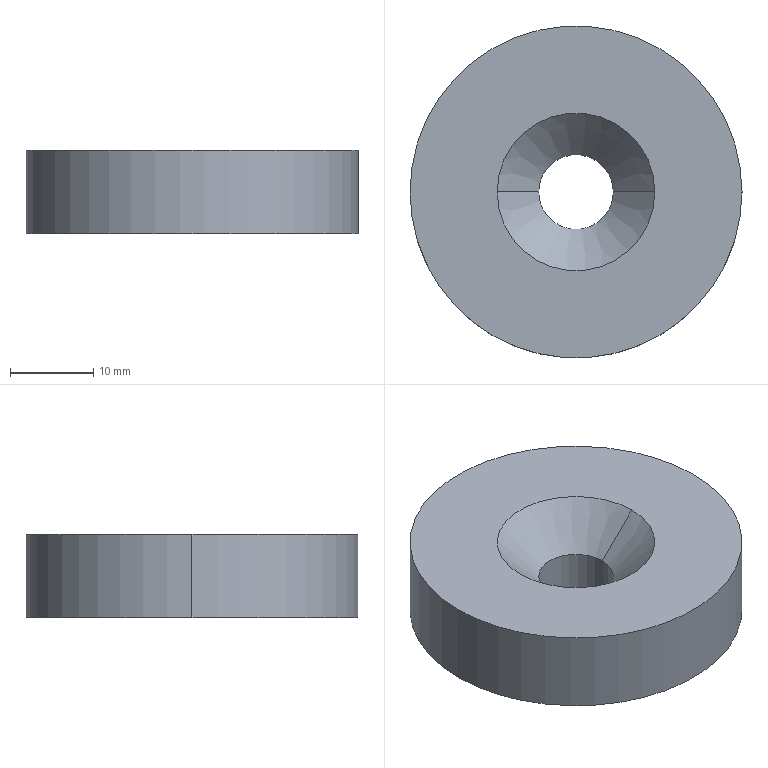Part | SolidWorks | features BaseBody 1 | 1 solid | 8 faces | box 40 x 40 x 10 mm | volume 11446 mm3 | cylinder 4 | cone 2 | plane 2 | commonest cylinder face diameters 9 x2 40 x2
STEP:
#1=CARTESIAN_POINT('',(-4.5,-165.,-385.5));
#2=VERTEX_POINT('',#1);
#3=CARTESIAN_POINT('',(4.5,-165.,-385.5));
#4=VERTEX_POINT('',#3);
#5=CARTESIAN_POINT('',(0.,-165.,-385.5));
#6=DIRECTION('',(0.,0.,1.));
#7=DIRECTION('',(-1.,0.,0.));
#8=AXIS2_PLACEMENT_3D('',#5,#6,#7);
#9=CIRCLE('',#8,4.5);
#10=EDGE_CURVE('',#2,#4,#9,.T.);
#11=ORIENTED_EDGE('',*,*,#10,.F.);
#12=CARTESIAN_POINT('',(-9.5,-165.,-380.5));
#13=VERTEX_POINT('',#12);
#14=CARTESIAN_POINT('',(-4.5,-165.,-385.5));
#15=DIRECTION('',(-0.7071,0.,0.7071));
#16=VECTOR('',#15,1000.);
#17=LINE('',#14,#16);
#18=EDGE_CURVE('',#2,#13,#17,.T.);
#19=ORIENTED_EDGE('',*,*,#18,.T.);
#20=CARTESIAN_POINT('',(9.5,-165.,-380.5));
#21=VERTEX_POINT('',#20);
#22=CARTESIAN_POINT('',(0.,-165.,-380.5));
#23=DIRECTION('',(0.,0.,1.));
#24=DIRECTION('',(-1.,0.,0.));
#25=AXIS2_PLACEMENT_3D('',#22,#23,#24);
#26=CIRCLE('',#25,9.5);
#27=EDGE_CURVE('',#13,#21,#26,.T.);
#28=ORIENTED_EDGE('',*,*,#27,.T.);
#29=CARTESIAN_POINT('',(4.5,-165.,-385.5));
#30=DIRECTION('',(0.7071,0.,0.7071));
#31=VECTOR('',#30,1000.);
#32=LINE('',#29,#31);
#33=EDGE_CURVE('',#4,#21,#32,.T.);
#34=ORIENTED_EDGE('',*,*,#33,.F.);
#35=EDGE_LOOP('',(#11,#19,#28,#34));
#36=FACE_OUTER_BOUND('',#35,.T.);
#37=CARTESIAN_POINT('',(0.,-165.,-385.5));
#38=DIRECTION('',(0.,0.,1.));
#39=DIRECTION('',(1.,0.,0.));
#40=AXIS2_PLACEMENT_3D('',#37,#38,#39);
#41=CONICAL_SURFACE('',#40,4.5,0.7854);
#42=ADVANCED_FACE('',(#36),#41,.F.);
#43=CARTESIAN_POINT('',(0.,-165.,-385.5));
#44=DIRECTION('',(0.,0.,1.));
#45=DIRECTION('',(-1.,0.,0.));
#46=AXIS2_PLACEMENT_3D('',#43,#44,#45);
#47=CIRCLE('',#46,4.5);
#48=EDGE_CURVE('',#4,#2,#47,.T.);
#49=ORIENTED_EDGE('',*,*,#48,.T.);
#50=CARTESIAN_POINT('',(-4.5,-165.,-390.5));
#51=VERTEX_POINT('',#50);
#52=CARTESIAN_POINT('',(-4.5,-165.,-380.5));
#53=DIRECTION('',(0.,0.,-1.));
#54=VECTOR('',#53,1000.);
#55=LINE('',#52,#54);
#56=EDGE_CURVE('',#2,#51,#55,.T.);
#57=ORIENTED_EDGE('',*,*,#56,.T.);
#58=CARTESIAN_POINT('',(4.5,-165.,-390.5));
#59=VERTEX_POINT('',#58);
#60=CARTESIAN_POINT('',(0.,-165.,-390.5));
#61=DIRECTION('',(0.,0.,-1.));
#62=DIRECTION('',(-1.,0.,0.));
#63=AXIS2_PLACEMENT_3D('',#60,#61,#62);
#64=CIRCLE('',#63,4.5);
#65=EDGE_CURVE('',#51,#59,#64,.T.);
#66=ORIENTED_EDGE('',*,*,#65,.T.);
#67=CARTESIAN_POINT('',(4.5,-165.,-380.5));
#68=DIRECTION('',(0.,0.,-1.));
#69=VECTOR('',#68,1000.);
#70=LINE('',#67,#69);
#71=EDGE_CURVE('',#4,#59,#70,.T.);
#72=ORIENTED_EDGE('',*,*,#71,.F.);
#73=EDGE_LOOP('',(#49,#57,#66,#72));
#74=FACE_OUTER_BOUND('',#73,.T.);
#75=CARTESIAN_POINT('',(0.,-165.,-380.5));
#76=DIRECTION('',(0.,0.,-1.));
#77=DIRECTION('',(1.,0.,0.));
#78=AXIS2_PLACEMENT_3D('',#75,#76,#77);
#79=CYLINDRICAL_SURFACE('',#78,4.5);
#80=ADVANCED_FACE('',(#74),#79,.F.);
#81=CARTESIAN_POINT('',(20.,-165.,-390.5));
#82=VERTEX_POINT('',#81);
#83=CARTESIAN_POINT('',(-20.,-165.,-390.5));
#84=VERTEX_POINT('',#83);
#85=CARTESIAN_POINT('',(0.,-165.,-390.5));
#86=DIRECTION('',(0.,0.,-1.));
#87=DIRECTION('',(0.,1.,0.));
#88=AXIS2_PLACEMENT_3D('',#85,#86,#87);
#89=CIRCLE('',#88,20.);
#90=EDGE_CURVE('',#82,#84,#89,.T.);
#91=ORIENTED_EDGE('',*,*,#90,.F.);
#92=CARTESIAN_POINT('',(20.,-165.,-380.5));
#93=VERTEX_POINT('',#92);
#94=CARTESIAN_POINT('',(20.,-165.,-390.5));
#95=DIRECTION('',(0.,0.,1.));
#96=VECTOR('',#95,1000.);
#97=LINE('',#94,#96);
#98=EDGE_CURVE('',#82,#93,#97,.T.);
#99=ORIENTED_EDGE('',*,*,#98,.T.);
#100=CARTESIAN_POINT('',(-20.,-165.,-380.5));
#101=VERTEX_POINT('',#100);
#102=CARTESIAN_POINT('',(0.,-165.,-380.5));
#103=DIRECTION('',(0.,0.,-1.));
#104=DIRECTION('',(0.,1.,0.));
#105=AXIS2_PLACEMENT_3D('',#102,#103,#104);
#106=CIRCLE('',#105,20.);
#107=EDGE_CURVE('',#93,#101,#106,.T.);
#108=ORIENTED_EDGE('',*,*,#107,.T.);
#109=CARTESIAN_POINT('',(-20.,-165.,-390.5));
#110=DIRECTION('',(0.,0.,1.));
#111=VECTOR('',#110,1000.);
#112=LINE('',#109,#111);
#113=EDGE_CURVE('',#84,#101,#112,.T.);
#114=ORIENTED_EDGE('',*,*,#113,.F.);
#115=EDGE_LOOP('',(#91,#99,#108,#114));
#116=FACE_OUTER_BOUND('',#115,.T.);
#117=CARTESIAN_POINT('',(0.,-165.,-390.5));
#118=DIRECTION('',(0.,0.,1.));
#119=DIRECTION('',(-1.,0.,0.));
#120=AXIS2_PLACEMENT_3D('',#117,#118,#119);
#121=CYLINDRICAL_SURFACE('',#120,20.);
#122=ADVANCED_FACE('',(#116),#121,.T.);
#123=ORIENTED_EDGE('',*,*,#98,.F.);
#124=CARTESIAN_POINT('',(0.,-165.,-390.5));
#125=DIRECTION('',(0.,0.,-1.));
#126=DIRECTION('',(0.,1.,0.));
#127=AXIS2_PLACEMENT_3D('',#124,#125,#126);
#128=CIRCLE('',#127,20.);
#129=EDGE_CURVE('',#84,#82,#128,.T.);
#130=ORIENTED_EDGE('',*,*,#129,.F.);
#131=ORIENTED_EDGE('',*,*,#113,.T.);
#132=CARTESIAN_POINT('',(0.,-165.,-380.5));
#133=DIRECTION('',(0.,0.,-1.));
#134=DIRECTION('',(0.,1.,0.));
#135=AXIS2_PLACEMENT_3D('',#132,#133,#134);
#136=CIRCLE('',#135,20.);
#137=EDGE_CURVE('',#101,#93,#136,.T.);
#138=ORIENTED_EDGE('',*,*,#137,.T.);
#139=EDGE_LOOP('',(#123,#130,#131,#138));
#140=FACE_OUTER_BOUND('',#139,.T.);
#141=CARTESIAN_POINT('',(0.,-165.,-390.5));
#142=DIRECTION('',(0.,0.,1.));
#143=DIRECTION('',(-1.,0.,0.));
#144=AXIS2_PLACEMENT_3D('',#141,#142,#143);
#145=CYLINDRICAL_SURFACE('',#144,20.);
#146=ADVANCED_FACE('',(#140),#145,.T.);
#147=ORIENTED_EDGE('',*,*,#56,.F.);
#148=ORIENTED_EDGE('',*,*,#10,.T.);
#149=ORIENTED_EDGE('',*,*,#71,.T.);
#150=CARTESIAN_POINT('',(0.,-165.,-390.5));
#151=DIRECTION('',(0.,0.,-1.));
#152=DIRECTION('',(-1.,0.,0.));
#153=AXIS2_PLACEMENT_3D('',#150,#151,#152);
#154=CIRCLE('',#153,4.5);
#155=EDGE_CURVE('',#59,#51,#154,.T.);
#156=ORIENTED_EDGE('',*,*,#155,.T.);
#157=EDGE_LOOP('',(#147,#148,#149,#156));
#158=FACE_OUTER_BOUND('',#157,.T.);
#159=CARTESIAN_POINT('',(0.,-165.,-380.5));
#160=DIRECTION('',(0.,0.,-1.));
#161=DIRECTION('',(1.,0.,0.));
#162=AXIS2_PLACEMENT_3D('',#159,#160,#161);
#163=CYLINDRICAL_SURFACE('',#162,4.5);
#164=ADVANCED_FACE('',(#158),#163,.F.);
#165=ORIENTED_EDGE('',*,*,#155,.F.);
#166=ORIENTED_EDGE('',*,*,#65,.F.);
#167=EDGE_LOOP('',(#165,#166));
#168=FACE_BOUND('',#167,.T.);
#169=ORIENTED_EDGE('',*,*,#129,.T.);
#170=ORIENTED_EDGE('',*,*,#90,.T.);
#171=EDGE_LOOP('',(#169,#170));
#172=FACE_OUTER_BOUND('',#171,.T.);
#173=CARTESIAN_POINT('',(0.,-165.,-390.5));
#174=DIRECTION('',(0.,0.,1.));
#175=DIRECTION('',(-1.,0.,0.));
#176=AXIS2_PLACEMENT_3D('',#173,#174,#175);
#177=PLANE('',#176);
#178=ADVANCED_FACE('',(#168,#172),#177,.F.);
#179=CARTESIAN_POINT('',(0.,-165.,-380.5));
#180=DIRECTION('',(0.,0.,1.));
#181=DIRECTION('',(-1.,0.,0.));
#182=AXIS2_PLACEMENT_3D('',#179,#180,#181);
#183=CIRCLE('',#182,9.5);
#184=EDGE_CURVE('',#21,#13,#183,.T.);
#185=ORIENTED_EDGE('',*,*,#184,.F.);
#186=ORIENTED_EDGE('',*,*,#27,.F.);
#187=EDGE_LOOP('',(#185,#186));
#188=FACE_BOUND('',#187,.T.);
#189=ORIENTED_EDGE('',*,*,#137,.F.);
#190=ORIENTED_EDGE('',*,*,#107,.F.);
#191=EDGE_LOOP('',(#189,#190));
#192=FACE_OUTER_BOUND('',#191,.T.);
#193=CARTESIAN_POINT('',(0.,-165.,-380.5));
#194=DIRECTION('',(0.,0.,1.));
#195=DIRECTION('',(-1.,0.,0.));
#196=AXIS2_PLACEMENT_3D('',#193,#194,#195);
#197=PLANE('',#196);
#198=ADVANCED_FACE('',(#188,#192),#197,.T.);
#199=ORIENTED_EDGE('',*,*,#18,.F.);
#200=ORIENTED_EDGE('',*,*,#48,.F.);
#201=ORIENTED_EDGE('',*,*,#33,.T.);
#202=ORIENTED_EDGE('',*,*,#184,.T.);
#203=EDGE_LOOP('',(#199,#200,#201,#202));
#204=FACE_OUTER_BOUND('',#203,.T.);
#205=CARTESIAN_POINT('',(0.,-165.,-385.5));
#206=DIRECTION('',(0.,0.,1.));
#207=DIRECTION('',(1.,0.,0.));
#208=AXIS2_PLACEMENT_3D('',#205,#206,#207);
#209=CONICAL_SURFACE('',#208,4.5,0.7854);
#210=ADVANCED_FACE('',(#204),#209,.F.);
#211=CLOSED_SHELL('',(#42,#80,#122,#146,#164,#178,#198,#210));
#212=MANIFOLD_SOLID_BREP('',#211);
#213=CARTESIAN_POINT('',(0.,0.,0.));
#214=DIRECTION('',(0.,0.,1.));
#215=DIRECTION('',(1.,0.,0.));
#216=AXIS2_PLACEMENT_3D('',#213,#214,#215);
#217=(LENGTH_UNIT()NAMED_UNIT(*)SI_UNIT(.MILLI.,.METRE.));
#218=UNCERTAINTY_MEASURE_WITH_UNIT(LENGTH_MEASURE(0.00001),#217,'','');
#219=(NAMED_UNIT(*)PLANE_ANGLE_UNIT()SI_UNIT($,.RADIAN.));
#220=(NAMED_UNIT(*)SI_UNIT($,.STERADIAN.)SOLID_ANGLE_UNIT());
#221=(GEOMETRIC_REPRESENTATION_CONTEXT(3)GLOBAL_UNCERTAINTY_ASSIGNED_CONTEXT((#218))GLOBAL_UNIT_ASSIGNED_CONTEXT((#217,#219,#220))REPRESENTATION_CONTEXT('',''));
#222=ADVANCED_BREP_SHAPE_REPRESENTATION('',(#212,#216),#221);